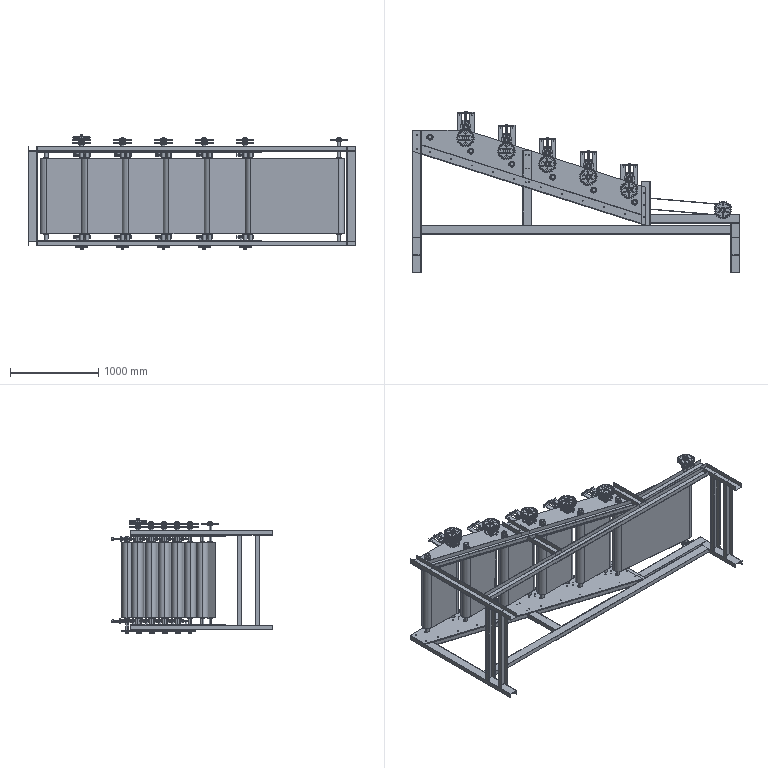Part | SolidWorks | features ReferencePattern 142, LocalLPattern 5, CompositeCurve 3, MirrorCompFeat 3, AEMSimFeature 1, LocalSketchPattern 1 | 169 solids | 9494 faces | volume 262282072 mm3 | cylinder 4772 | plane 2644 | torus 820 | cone 616 | spline 446 | sphere 196 | commonest cylinder face diameters 23.032 x588 41.467 x576 16.059 x360 198 x276 133.882 x230 109.368 x220